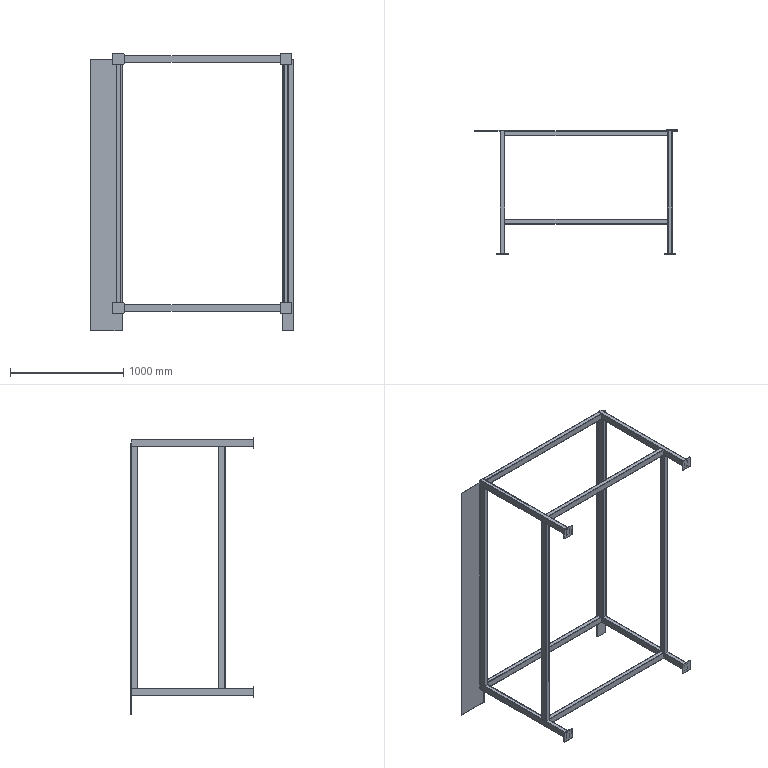Part | SolidWorks | features ICE 8, Extrusion 1 | 14 solids | 272 faces | box 1794 x 1094 x 2450 mm | volume 14966587 mm3 | plane 160 | cylinder 112 | commonest cylinder face diameters 0.2 x48 6 x48 20 x16